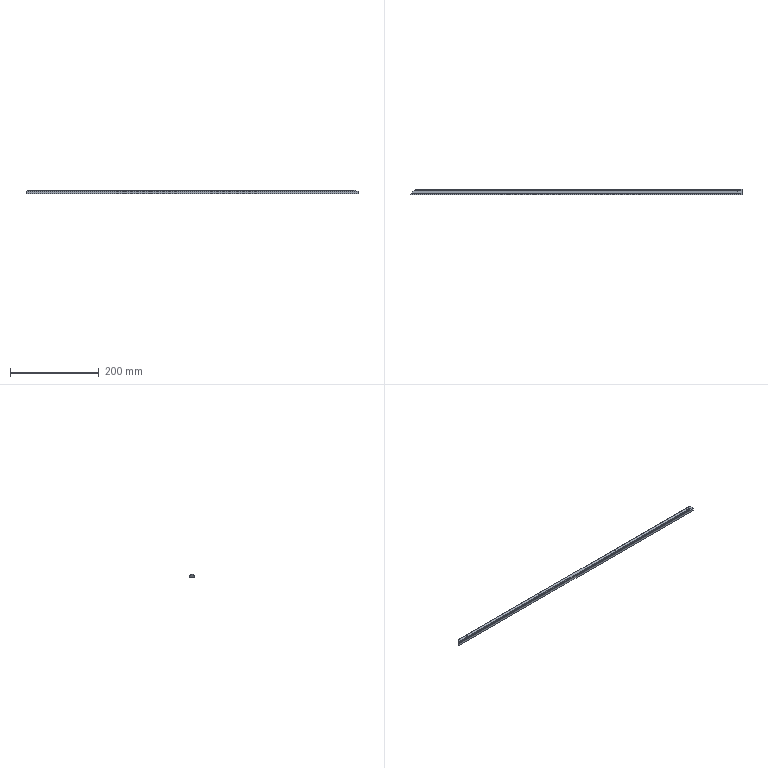Part | STEP file | J013-EBZ05-07-06 | 1 solid | 41 faces | box 748 x 12 x 8 mm | volume 60789 mm3 | plane 17 | cylinder 16 | cone 8 | commonest cylinder face diameters 3.24 x8 4 x8
STEP:
#1=CARTESIAN_POINT('',(257.5,6.,7.835));
#2=VERTEX_POINT('',#1);
#3=CARTESIAN_POINT('',(259.12,6.,6.9));
#4=VERTEX_POINT('',#3);
#5=CARTESIAN_POINT('',(259.12,6.,6.9));
#6=DIRECTION('',(0.866,0.,-0.5));
#7=VECTOR('',#6,1000.);
#8=LINE('',#5,#7);
#9=EDGE_CURVE('',#2,#4,#8,.T.);
#10=ORIENTED_EDGE('',*,*,#9,.F.);
#11=CARTESIAN_POINT('',(255.88,6.,6.9));
#12=VERTEX_POINT('',#11);
#13=CARTESIAN_POINT('',(255.88,6.,6.9));
#14=DIRECTION('',(-0.866,0.,-0.5));
#15=VECTOR('',#14,1000.);
#16=LINE('',#13,#15);
#17=EDGE_CURVE('',#2,#12,#16,.T.);
#18=ORIENTED_EDGE('',*,*,#17,.T.);
#19=CARTESIAN_POINT('',(257.5,6.,6.9));
#20=DIRECTION('',(0.,0.,-1.));
#21=DIRECTION('',(1.,0.,0.));
#22=AXIS2_PLACEMENT_3D('',#19,#20,#21);
#23=CIRCLE('',#22,1.62);
#24=EDGE_CURVE('',#12,#4,#23,.T.);
#25=ORIENTED_EDGE('',*,*,#24,.T.);
#26=EDGE_LOOP('',(#10,#18,#25));
#27=FACE_OUTER_BOUND('',#26,.T.);
#28=CARTESIAN_POINT('',(257.5,6.,6.9));
#29=DIRECTION('',(0.,0.,-1.));
#30=DIRECTION('',(1.,0.,0.));
#31=AXIS2_PLACEMENT_3D('',#28,#29,#30);
#32=CONICAL_SURFACE('',#31,1.62,1.047);
#33=ADVANCED_FACE('',(#27),#32,.F.);
#34=ORIENTED_EDGE('',*,*,#24,.F.);
#35=CARTESIAN_POINT('',(255.88,6.,6.));
#36=VERTEX_POINT('',#35);
#37=CARTESIAN_POINT('',(255.88,6.,0.));
#38=DIRECTION('',(0.,0.,-1.));
#39=VECTOR('',#38,1000.);
#40=LINE('',#37,#39);
#41=EDGE_CURVE('',#12,#36,#40,.T.);
#42=ORIENTED_EDGE('',*,*,#41,.T.);
#43=CARTESIAN_POINT('',(259.12,6.,6.));
#44=VERTEX_POINT('',#43);
#45=CARTESIAN_POINT('',(257.5,6.,6.));
#46=DIRECTION('',(0.,0.,-1.));
#47=DIRECTION('',(1.,0.,0.));
#48=AXIS2_PLACEMENT_3D('',#45,#46,#47);
#49=CIRCLE('',#48,1.62);
#50=EDGE_CURVE('',#36,#44,#49,.T.);
#51=ORIENTED_EDGE('',*,*,#50,.T.);
#52=CARTESIAN_POINT('',(259.12,6.,0.));
#53=DIRECTION('',(0.,0.,-1.));
#54=VECTOR('',#53,1000.);
#55=LINE('',#52,#54);
#56=EDGE_CURVE('',#4,#44,#55,.T.);
#57=ORIENTED_EDGE('',*,*,#56,.F.);
#58=EDGE_LOOP('',(#34,#42,#51,#57));
#59=FACE_OUTER_BOUND('',#58,.T.);
#60=CARTESIAN_POINT('',(257.5,6.,0.));
#61=DIRECTION('',(0.,0.,-1.));
#62=DIRECTION('',(1.,0.,0.));
#63=AXIS2_PLACEMENT_3D('',#60,#61,#62);
#64=CYLINDRICAL_SURFACE('',#63,1.62);
#65=ADVANCED_FACE('',(#59),#64,.F.);
#66=CARTESIAN_POINT('',(255.5,6.,6.));
#67=VERTEX_POINT('',#66);
#68=CARTESIAN_POINT('',(259.5,6.,6.));
#69=VERTEX_POINT('',#68);
#70=CARTESIAN_POINT('',(257.5,6.,6.));
#71=DIRECTION('',(0.,0.,-1.));
#72=DIRECTION('',(1.,0.,0.));
#73=AXIS2_PLACEMENT_3D('',#70,#71,#72);
#74=CIRCLE('',#73,2.);
#75=EDGE_CURVE('',#67,#69,#74,.T.);
#76=ORIENTED_EDGE('',*,*,#75,.F.);
#77=CARTESIAN_POINT('',(255.5,6.,0.));
#78=VERTEX_POINT('',#77);
#79=CARTESIAN_POINT('',(255.5,6.,0.));
#80=DIRECTION('',(0.,0.,-1.));
#81=VECTOR('',#80,1000.);
#82=LINE('',#79,#81);
#83=EDGE_CURVE('',#67,#78,#82,.T.);
#84=ORIENTED_EDGE('',*,*,#83,.T.);
#85=CARTESIAN_POINT('',(259.5,6.,0.));
#86=VERTEX_POINT('',#85);
#87=CARTESIAN_POINT('',(257.5,6.,0.));
#88=DIRECTION('',(0.,0.,-1.));
#89=DIRECTION('',(1.,0.,0.));
#90=AXIS2_PLACEMENT_3D('',#87,#88,#89);
#91=CIRCLE('',#90,2.);
#92=EDGE_CURVE('',#78,#86,#91,.T.);
#93=ORIENTED_EDGE('',*,*,#92,.T.);
#94=CARTESIAN_POINT('',(259.5,6.,0.));
#95=DIRECTION('',(0.,0.,-1.));
#96=VECTOR('',#95,1000.);
#97=LINE('',#94,#96);
#98=EDGE_CURVE('',#69,#86,#97,.T.);
#99=ORIENTED_EDGE('',*,*,#98,.F.);
#100=EDGE_LOOP('',(#76,#84,#93,#99));
#101=FACE_OUTER_BOUND('',#100,.T.);
#102=CARTESIAN_POINT('',(257.5,6.,0.));
#103=DIRECTION('',(0.,0.,-1.));
#104=DIRECTION('',(1.,0.,0.));
#105=AXIS2_PLACEMENT_3D('',#102,#103,#104);
#106=CYLINDRICAL_SURFACE('',#105,2.);
#107=ADVANCED_FACE('',(#101),#106,.F.);
#108=CARTESIAN_POINT('',(497.5,6.,7.835));
#109=VERTEX_POINT('',#108);
#110=CARTESIAN_POINT('',(499.12,6.,6.9));
#111=VERTEX_POINT('',#110);
#112=CARTESIAN_POINT('',(499.12,6.,6.9));
#113=DIRECTION('',(0.866,0.,-0.5));
#114=VECTOR('',#113,1000.);
#115=LINE('',#112,#114);
#116=EDGE_CURVE('',#109,#111,#115,.T.);
#117=ORIENTED_EDGE('',*,*,#116,.F.);
#118=CARTESIAN_POINT('',(495.88,6.,6.9));
#119=VERTEX_POINT('',#118);
#120=CARTESIAN_POINT('',(495.88,6.,6.9));
#121=DIRECTION('',(-0.866,0.,-0.5));
#122=VECTOR('',#121,1000.);
#123=LINE('',#120,#122);
#124=EDGE_CURVE('',#109,#119,#123,.T.);
#125=ORIENTED_EDGE('',*,*,#124,.T.);
#126=CARTESIAN_POINT('',(497.5,6.,6.9));
#127=DIRECTION('',(0.,0.,-1.));
#128=DIRECTION('',(1.,0.,0.));
#129=AXIS2_PLACEMENT_3D('',#126,#127,#128);
#130=CIRCLE('',#129,1.62);
#131=EDGE_CURVE('',#119,#111,#130,.T.);
#132=ORIENTED_EDGE('',*,*,#131,.T.);
#133=EDGE_LOOP('',(#117,#125,#132));
#134=FACE_OUTER_BOUND('',#133,.T.);
#135=CARTESIAN_POINT('',(497.5,6.,6.9));
#136=DIRECTION('',(0.,0.,-1.));
#137=DIRECTION('',(1.,0.,0.));
#138=AXIS2_PLACEMENT_3D('',#135,#136,#137);
#139=CONICAL_SURFACE('',#138,1.62,1.047);
#140=ADVANCED_FACE('',(#134),#139,.F.);
#141=ORIENTED_EDGE('',*,*,#131,.F.);
#142=CARTESIAN_POINT('',(495.88,6.,6.));
#143=VERTEX_POINT('',#142);
#144=CARTESIAN_POINT('',(495.88,6.,0.));
#145=DIRECTION('',(0.,0.,-1.));
#146=VECTOR('',#145,1000.);
#147=LINE('',#144,#146);
#148=EDGE_CURVE('',#119,#143,#147,.T.);
#149=ORIENTED_EDGE('',*,*,#148,.T.);
#150=CARTESIAN_POINT('',(499.12,6.,6.));
#151=VERTEX_POINT('',#150);
#152=CARTESIAN_POINT('',(497.5,6.,6.));
#153=DIRECTION('',(0.,0.,-1.));
#154=DIRECTION('',(1.,0.,0.));
#155=AXIS2_PLACEMENT_3D('',#152,#153,#154);
#156=CIRCLE('',#155,1.62);
#157=EDGE_CURVE('',#143,#151,#156,.T.);
#158=ORIENTED_EDGE('',*,*,#157,.T.);
#159=CARTESIAN_POINT('',(499.12,6.,0.));
#160=DIRECTION('',(0.,0.,-1.));
#161=VECTOR('',#160,1000.);
#162=LINE('',#159,#161);
#163=EDGE_CURVE('',#111,#151,#162,.T.);
#164=ORIENTED_EDGE('',*,*,#163,.F.);
#165=EDGE_LOOP('',(#141,#149,#158,#164));
#166=FACE_OUTER_BOUND('',#165,.T.);
#167=CARTESIAN_POINT('',(497.5,6.,0.));
#168=DIRECTION('',(0.,0.,-1.));
#169=DIRECTION('',(1.,0.,0.));
#170=AXIS2_PLACEMENT_3D('',#167,#168,#169);
#171=CYLINDRICAL_SURFACE('',#170,1.62);
#172=ADVANCED_FACE('',(#166),#171,.F.);
#173=CARTESIAN_POINT('',(495.5,6.,6.));
#174=VERTEX_POINT('',#173);
#175=CARTESIAN_POINT('',(499.5,6.,6.));
#176=VERTEX_POINT('',#175);
#177=CARTESIAN_POINT('',(497.5,6.,6.));
#178=DIRECTION('',(0.,0.,-1.));
#179=DIRECTION('',(1.,0.,0.));
#180=AXIS2_PLACEMENT_3D('',#177,#178,#179);
#181=CIRCLE('',#180,2.);
#182=EDGE_CURVE('',#174,#176,#181,.T.);
#183=ORIENTED_EDGE('',*,*,#182,.F.);
#184=CARTESIAN_POINT('',(495.5,6.,0.));
#185=VERTEX_POINT('',#184);
#186=CARTESIAN_POINT('',(495.5,6.,0.));
#187=DIRECTION('',(0.,0.,-1.));
#188=VECTOR('',#187,1000.);
#189=LINE('',#186,#188);
#190=EDGE_CURVE('',#174,#185,#189,.T.);
#191=ORIENTED_EDGE('',*,*,#190,.T.);
#192=CARTESIAN_POINT('',(499.5,6.,0.));
#193=VERTEX_POINT('',#192);
#194=CARTESIAN_POINT('',(497.5,6.,0.));
#195=DIRECTION('',(0.,0.,-1.));
#196=DIRECTION('',(1.,0.,0.));
#197=AXIS2_PLACEMENT_3D('',#194,#195,#196);
#198=CIRCLE('',#197,2.);
#199=EDGE_CURVE('',#185,#193,#198,.T.);
#200=ORIENTED_EDGE('',*,*,#199,.T.);
#201=CARTESIAN_POINT('',(499.5,6.,0.));
#202=DIRECTION('',(0.,0.,-1.));
#203=VECTOR('',#202,1000.);
#204=LINE('',#201,#203);
#205=EDGE_CURVE('',#176,#193,#204,.T.);
#206=ORIENTED_EDGE('',*,*,#205,.F.);
#207=EDGE_LOOP('',(#183,#191,#200,#206));
#208=FACE_OUTER_BOUND('',#207,.T.);
#209=CARTESIAN_POINT('',(497.5,6.,0.));
#210=DIRECTION('',(0.,0.,-1.));
#211=DIRECTION('',(1.,0.,0.));
#212=AXIS2_PLACEMENT_3D('',#209,#210,#211);
#213=CYLINDRICAL_SURFACE('',#212,2.);
#214=ADVANCED_FACE('',(#208),#213,.F.);
#215=CARTESIAN_POINT('',(27.5,6.,7.835));
#216=VERTEX_POINT('',#215);
#217=CARTESIAN_POINT('',(29.12,6.,6.9));
#218=VERTEX_POINT('',#217);
#219=CARTESIAN_POINT('',(29.12,6.,6.9));
#220=DIRECTION('',(0.866,0.,-0.5));
#221=VECTOR('',#220,1000.);
#222=LINE('',#219,#221);
#223=EDGE_CURVE('',#216,#218,#222,.T.);
#224=ORIENTED_EDGE('',*,*,#223,.F.);
#225=CARTESIAN_POINT('',(25.88,6.,6.9));
#226=VERTEX_POINT('',#225);
#227=CARTESIAN_POINT('',(25.88,6.,6.9));
#228=DIRECTION('',(-0.866,0.,-0.5));
#229=VECTOR('',#228,1000.);
#230=LINE('',#227,#229);
#231=EDGE_CURVE('',#216,#226,#230,.T.);
#232=ORIENTED_EDGE('',*,*,#231,.T.);
#233=CARTESIAN_POINT('',(27.5,6.,6.9));
#234=DIRECTION('',(0.,0.,-1.));
#235=DIRECTION('',(1.,0.,0.));
#236=AXIS2_PLACEMENT_3D('',#233,#234,#235);
#237=CIRCLE('',#236,1.62);
#238=EDGE_CURVE('',#226,#218,#237,.T.);
#239=ORIENTED_EDGE('',*,*,#238,.T.);
#240=EDGE_LOOP('',(#224,#232,#239));
#241=FACE_OUTER_BOUND('',#240,.T.);
#242=CARTESIAN_POINT('',(27.5,6.,6.9));
#243=DIRECTION('',(0.,0.,-1.));
#244=DIRECTION('',(1.,0.,0.));
#245=AXIS2_PLACEMENT_3D('',#242,#243,#244);
#246=CONICAL_SURFACE('',#245,1.62,1.047);
#247=ADVANCED_FACE('',(#241),#246,.F.);
#248=ORIENTED_EDGE('',*,*,#238,.F.);
#249=CARTESIAN_POINT('',(25.88,6.,6.));
#250=VERTEX_POINT('',#249);
#251=CARTESIAN_POINT('',(25.88,6.,0.));
#252=DIRECTION('',(0.,0.,-1.));
#253=VECTOR('',#252,1000.);
#254=LINE('',#251,#253);
#255=EDGE_CURVE('',#226,#250,#254,.T.);
#256=ORIENTED_EDGE('',*,*,#255,.T.);
#257=CARTESIAN_POINT('',(29.12,6.,6.));
#258=VERTEX_POINT('',#257);
#259=CARTESIAN_POINT('',(27.5,6.,6.));
#260=DIRECTION('',(0.,0.,-1.));
#261=DIRECTION('',(1.,0.,0.));
#262=AXIS2_PLACEMENT_3D('',#259,#260,#261);
#263=CIRCLE('',#262,1.62);
#264=EDGE_CURVE('',#250,#258,#263,.T.);
#265=ORIENTED_EDGE('',*,*,#264,.T.);
#266=CARTESIAN_POINT('',(29.12,6.,0.));
#267=DIRECTION('',(0.,0.,-1.));
#268=VECTOR('',#267,1000.);
#269=LINE('',#266,#268);
#270=EDGE_CURVE('',#218,#258,#269,.T.);
#271=ORIENTED_EDGE('',*,*,#270,.F.);
#272=EDGE_LOOP('',(#248,#256,#265,#271));
#273=FACE_OUTER_BOUND('',#272,.T.);
#274=CARTESIAN_POINT('',(27.5,6.,0.));
#275=DIRECTION('',(0.,0.,-1.));
#276=DIRECTION('',(1.,0.,0.));
#277=AXIS2_PLACEMENT_3D('',#274,#275,#276);
#278=CYLINDRICAL_SURFACE('',#277,1.62);
#279=ADVANCED_FACE('',(#273),#278,.F.);
#280=CARTESIAN_POINT('',(25.5,6.,6.));
#281=VERTEX_POINT('',#280);
#282=CARTESIAN_POINT('',(29.5,6.,6.));
#283=VERTEX_POINT('',#282);
#284=CARTESIAN_POINT('',(27.5,6.,6.));
#285=DIRECTION('',(0.,0.,-1.));
#286=DIRECTION('',(1.,0.,0.));
#287=AXIS2_PLACEMENT_3D('',#284,#285,#286);
#288=CIRCLE('',#287,2.);
#289=EDGE_CURVE('',#281,#283,#288,.T.);
#290=ORIENTED_EDGE('',*,*,#289,.F.);
#291=CARTESIAN_POINT('',(25.5,6.,0.));
#292=VERTEX_POINT('',#291);
#293=CARTESIAN_POINT('',(25.5,6.,0.));
#294=DIRECTION('',(0.,0.,-1.));
#295=VECTOR('',#294,1000.);
#296=LINE('',#293,#295);
#297=EDGE_CURVE('',#281,#292,#296,.T.);
#298=ORIENTED_EDGE('',*,*,#297,.T.);
#299=CARTESIAN_POINT('',(29.5,6.,0.));
#300=VERTEX_POINT('',#299);
#301=CARTESIAN_POINT('',(27.5,6.,0.));
#302=DIRECTION('',(0.,0.,-1.));
#303=DIRECTION('',(1.,0.,0.));
#304=AXIS2_PLACEMENT_3D('',#301,#302,#303);
#305=CIRCLE('',#304,2.);
#306=EDGE_CURVE('',#292,#300,#305,.T.);
#307=ORIENTED_EDGE('',*,*,#306,.T.);
#308=CARTESIAN_POINT('',(29.5,6.,0.));
#309=DIRECTION('',(0.,0.,-1.));
#310=VECTOR('',#309,1000.);
#311=LINE('',#308,#310);
#312=EDGE_CURVE('',#283,#300,#311,.T.);
#313=ORIENTED_EDGE('',*,*,#312,.F.);
#314=EDGE_LOOP('',(#290,#298,#307,#313));
#315=FACE_OUTER_BOUND('',#314,.T.);
#316=CARTESIAN_POINT('',(27.5,6.,0.));
#317=DIRECTION('',(0.,0.,-1.));
#318=DIRECTION('',(1.,0.,0.));
#319=AXIS2_PLACEMENT_3D('',#316,#317,#318);
#320=CYLINDRICAL_SURFACE('',#319,2.);
#321=ADVANCED_FACE('',(#315),#320,.F.);
#322=CARTESIAN_POINT('',(727.5,6.,7.835));
#323=VERTEX_POINT('',#322);
#324=CARTESIAN_POINT('',(729.12,6.,6.9));
#325=VERTEX_POINT('',#324);
#326=CARTESIAN_POINT('',(729.12,6.,6.9));
#327=DIRECTION('',(0.866,0.,-0.5));
#328=VECTOR('',#327,1000.);
#329=LINE('',#326,#328);
#330=EDGE_CURVE('',#323,#325,#329,.T.);
#331=ORIENTED_EDGE('',*,*,#330,.F.);
#332=CARTESIAN_POINT('',(725.88,6.,6.9));
#333=VERTEX_POINT('',#332);
#334=CARTESIAN_POINT('',(725.88,6.,6.9));
#335=DIRECTION('',(-0.866,0.,-0.5));
#336=VECTOR('',#335,1000.);
#337=LINE('',#334,#336);
#338=EDGE_CURVE('',#323,#333,#337,.T.);
#339=ORIENTED_EDGE('',*,*,#338,.T.);
#340=CARTESIAN_POINT('',(727.5,6.,6.9));
#341=DIRECTION('',(0.,0.,-1.));
#342=DIRECTION('',(1.,0.,0.));
#343=AXIS2_PLACEMENT_3D('',#340,#341,#342);
#344=CIRCLE('',#343,1.62);
#345=EDGE_CURVE('',#333,#325,#344,.T.);
#346=ORIENTED_EDGE('',*,*,#345,.T.);
#347=EDGE_LOOP('',(#331,#339,#346));
#348=FACE_OUTER_BOUND('',#347,.T.);
#349=CARTESIAN_POINT('',(727.5,6.,6.9));
#350=DIRECTION('',(0.,0.,-1.));
#351=DIRECTION('',(1.,0.,0.));
#352=AXIS2_PLACEMENT_3D('',#349,#350,#351);
#353=CONICAL_SURFACE('',#352,1.62,1.047);
#354=ADVANCED_FACE('',(#348),#353,.F.);
#355=ORIENTED_EDGE('',*,*,#345,.F.);
#356=CARTESIAN_POINT('',(725.88,6.,6.));
#357=VERTEX_POINT('',#356);
#358=CARTESIAN_POINT('',(725.88,6.,0.));
#359=DIRECTION('',(0.,0.,-1.));
#360=VECTOR('',#359,1000.);
#361=LINE('',#358,#360);
#362=EDGE_CURVE('',#333,#357,#361,.T.);
#363=ORIENTED_EDGE('',*,*,#362,.T.);
#364=CARTESIAN_POINT('',(729.12,6.,6.));
#365=VERTEX_POINT('',#364);
#366=CARTESIAN_POINT('',(727.5,6.,6.));
#367=DIRECTION('',(0.,0.,-1.));
#368=DIRECTION('',(1.,0.,0.));
#369=AXIS2_PLACEMENT_3D('',#366,#367,#368);
#370=CIRCLE('',#369,1.62);
#371=EDGE_CURVE('',#357,#365,#370,.T.);
#372=ORIENTED_EDGE('',*,*,#371,.T.);
#373=CARTESIAN_POINT('',(729.12,6.,0.));
#374=DIRECTION('',(0.,0.,-1.));
#375=VECTOR('',#374,1000.);
#376=LINE('',#373,#375);
#377=EDGE_CURVE('',#325,#365,#376,.T.);
#378=ORIENTED_EDGE('',*,*,#377,.F.);
#379=EDGE_LOOP('',(#355,#363,#372,#378));
#380=FACE_OUTER_BOUND('',#379,.T.);
#381=CARTESIAN_POINT('',(727.5,6.,0.));
#382=DIRECTION('',(0.,0.,-1.));
#383=DIRECTION('',(1.,0.,0.));
#384=AXIS2_PLACEMENT_3D('',#381,#382,#383);
#385=CYLINDRICAL_SURFACE('',#384,1.62);
#386=ADVANCED_FACE('',(#380),#385,.F.);
#387=CARTESIAN_POINT('',(725.5,6.,6.));
#388=VERTEX_POINT('',#387);
#389=CARTESIAN_POINT('',(729.5,6.,6.));
#390=VERTEX_POINT('',#389);
#391=CARTESIAN_POINT('',(727.5,6.,6.));
#392=DIRECTION('',(0.,0.,-1.));
#393=DIRECTION('',(1.,0.,0.));
#394=AXIS2_PLACEMENT_3D('',#391,#392,#393);
#395=CIRCLE('',#394,2.);
#396=EDGE_CURVE('',#388,#390,#395,.T.);
#397=ORIENTED_EDGE('',*,*,#396,.F.);
#398=CARTESIAN_POINT('',(725.5,6.,0.));
#399=VERTEX_POINT('',#398);
#400=CARTESIAN_POINT('',(725.5,6.,0.));
#401=DIRECTION('',(0.,0.,-1.));
#402=VECTOR('',#401,1000.);
#403=LINE('',#400,#402);
#404=EDGE_CURVE('',#388,#399,#403,.T.);
#405=ORIENTED_EDGE('',*,*,#404,.T.);
#406=CARTESIAN_POINT('',(729.5,6.,0.));
#407=VERTEX_POINT('',#406);
#408=CARTESIAN_POINT('',(727.5,6.,0.));
#409=DIRECTION('',(0.,0.,-1.));
#410=DIRECTION('',(1.,0.,0.));
#411=AXIS2_PLACEMENT_3D('',#408,#409,#410);
#412=CIRCLE('',#411,2.);
#413=EDGE_CURVE('',#399,#407,#412,.T.);
#414=ORIENTED_EDGE('',*,*,#413,.T.);
#415=CARTESIAN_POINT('',(729.5,6.,0.));
#416=DIRECTION('',(0.,0.,-1.));
#417=VECTOR('',#416,1000.);
#418=LINE('',#415,#417);
#419=EDGE_CURVE('',#390,#407,#418,.T.);
#420=ORIENTED_EDGE('',*,*,#419,.F.);
#421=EDGE_LOOP('',(#397,#405,#414,#420));
#422=FACE_OUTER_BOUND('',#421,.T.);
#423=CARTESIAN_POINT('',(727.5,6.,0.));
#424=DIRECTION('',(0.,0.,-1.));
#425=DIRECTION('',(1.,0.,0.));
#426=AXIS2_PLACEMENT_3D('',#423,#424,#425);
#427=CYLINDRICAL_SURFACE('',#426,2.);
#428=ADVANCED_FACE('',(#422),#427,.F.);
#429=CARTESIAN_POINT('',(6.5,12.,5.5));
#430=VERTEX_POINT('',#429);
#431=CARTESIAN_POINT('',(742.5,12.,5.5));
#432=VERTEX_POINT('',#431);
#433=CARTESIAN_POINT('',(-5.5,12.,5.5));
#434=DIRECTION('',(1.,0.,0.));
#435=VECTOR('',#434,1000.);
#436=LINE('',#433,#435);
#437=EDGE_CURVE('',#430,#432,#436,.T.);
#438=ORIENTED_EDGE('',*,*,#437,.F.);
#439=CARTESIAN_POINT('',(3.8,9.3,5.5));
#440=VERTEX_POINT('',#439);
#441=CARTESIAN_POINT('',(-754.641,-749.141,5.5));
#442=DIRECTION('',(-0.7071,-0.7071,0.));
#443=VECTOR('',#442,1000.);
#444=LINE('',#441,#443);
#445=EDGE_CURVE('',#430,#440,#444,.T.);
#446=ORIENTED_EDGE('',*,*,#445,.T.);
#447=CARTESIAN_POINT('',(732.5,9.3,5.5));
#448=VERTEX_POINT('',#447);
#449=CARTESIAN_POINT('',(-5.5,9.3,5.5));
#450=DIRECTION('',(1.,0.,0.));
#451=VECTOR('',#450,1000.);
#452=LINE('',#449,#451);
#453=EDGE_CURVE('',#440,#448,#452,.T.);
#454=ORIENTED_EDGE('',*,*,#453,.T.);
#455=CARTESIAN_POINT('',(742.5,8.5,5.5));
#456=VERTEX_POINT('',#455);
#457=CARTESIAN_POINT('',(-185.364,82.729,5.5));
#458=DIRECTION('',(0.9968,-0.07975,0.));
#459=VECTOR('',#458,1000.);
#460=LINE('',#457,#459);
#461=EDGE_CURVE('',#448,#456,#460,.T.);
#462=ORIENTED_EDGE('',*,*,#461,.T.);
#463=CARTESIAN_POINT('',(742.5,12.,5.5));
#464=DIRECTION('',(0.,-1.,0.));
#465=VECTOR('',#464,1000.);
#466=LINE('',#463,#465);
#467=EDGE_CURVE('',#432,#456,#466,.T.);
#468=ORIENTED_EDGE('',*,*,#467,.F.);
#469=EDGE_LOOP('',(#438,#446,#454,#462,#468));
#470=FACE_OUTER_BOUND('',#469,.T.);
#471=CARTESIAN_POINT('',(-289.152,-1214.63,5.5));
#472=DIRECTION('',(0.,0.,-1.));
#473=DIRECTION('',(1.,0.,0.));
#474=AXIS2_PLACEMENT_3D('',#471,#472,#473);
#475=PLANE('',#474);
#476=ADVANCED_FACE('',(#470),#475,.F.);
#477=CARTESIAN_POINT('',(742.5,0.,5.5));
#478=VERTEX_POINT('',#477);
#479=CARTESIAN_POINT('',(-5.5,0.,5.5));
#480=VERTEX_POINT('',#479);
#481=CARTESIAN_POINT('',(742.5,0.,5.5));
#482=DIRECTION('',(-1.,0.,0.));
#483=VECTOR('',#482,1000.);
#484=LINE('',#481,#483);
#485=EDGE_CURVE('',#478,#480,#484,.T.);
#486=ORIENTED_EDGE('',*,*,#485,.T.);
#487=CARTESIAN_POINT('',(-5.5,0.,0.));
#488=VERTEX_POINT('',#487);
#489=CARTESIAN_POINT('',(-5.5,0.,0.));
#490=DIRECTION('',(0.,0.,1.));
#491=VECTOR('',#490,1000.);
#492=LINE('',#489,#491);
#493=EDGE_CURVE('',#488,#480,#492,.T.);
#494=ORIENTED_EDGE('',*,*,#493,.F.);
#495=CARTESIAN_POINT('',(742.5,0.,0.));
#496=VERTEX_POINT('',#495);
#497=CARTESIAN_POINT('',(742.5,0.,0.));
#498=DIRECTION('',(-1.,0.,0.));
#499=VECTOR('',#498,1000.);
#500=LINE('',#497,#499);
#501=EDGE_CURVE('',#496,#488,#500,.T.);
#502=ORIENTED_EDGE('',*,*,#501,.F.);
#503=CARTESIAN_POINT('',(742.5,0.,0.));
#504=DIRECTION('',(0.,0.,1.));
#505=VECTOR('',#504,1000.);
#506=LINE('',#503,#505);
#507=EDGE_CURVE('',#496,#478,#506,.T.);
#508=ORIENTED_EDGE('',*,*,#507,.T.);
#509=EDGE_LOOP('',(#486,#494,#502,#508));
#510=FACE_OUTER_BOUND('',#509,.T.);
#511=CARTESIAN_POINT('',(742.5,0.,0.));
#512=DIRECTION('',(0.,1.,0.));
#513=DIRECTION('',(0.,0.,1.));
#514=AXIS2_PLACEMENT_3D('',#511,#512,#513);
#515=PLANE('',#514);
#516=ADVANCED_FACE('',(#510),#515,.F.);
#517=CARTESIAN_POINT('',(6.5,12.,0.));
#518=VERTEX_POINT('',#517);
#519=CARTESIAN_POINT('',(742.5,12.,0.));
#520=VERTEX_POINT('',#519);
#521=CARTESIAN_POINT('',(-5.5,12.,0.));
#522=DIRECTION('',(1.,0.,0.));
#523=VECTOR('',#522,1000.);
#524=LINE('',#521,#523);
#525=EDGE_CURVE('',#518,#520,#524,.T.);
#526=ORIENTED_EDGE('',*,*,#525,.F.);
#527=CARTESIAN_POINT('',(6.5,12.,-0.001006));
#528=DIRECTION('',(0.,0.,1.));
#529=VECTOR('',#528,1000.);
#530=LINE('',#527,#529);
#531=EDGE_CURVE('',#518,#430,#530,.T.);
#532=ORIENTED_EDGE('',*,*,#531,.T.);
#533=ORIENTED_EDGE('',*,*,#437,.T.);
#534=CARTESIAN_POINT('',(742.5,12.,0.));
#535=DIRECTION('',(0.,0.,1.));
#536=VECTOR('',#535,1000.);
#537=LINE('',#534,#536);
#538=EDGE_CURVE('',#520,#432,#537,.T.);
#539=ORIENTED_EDGE('',*,*,#538,.F.);
#540=EDGE_LOOP('',(#526,#532,#533,#539));
#541=FACE_OUTER_BOUND('',#540,.T.);
#542=CARTESIAN_POINT('',(-5.5,12.,0.));
#543=DIRECTION('',(0.,-1.,0.));
#544=DIRECTION('',(0.,0.,-1.));
#545=AXIS2_PLACEMENT_3D('',#542,#543,#544);
#546=PLANE('',#545);
#547=ADVANCED_FACE('',(#541),#546,.F.);
#548=ORIENTED_EDGE('',*,*,#467,.T.);
#549=CARTESIAN_POINT('',(742.5,3.5,5.5));
#550=VERTEX_POINT('',#549);
#551=CARTESIAN_POINT('',(742.5,12.,5.5));
#552=DIRECTION('',(0.,-1.,0.));
#553=VECTOR('',#552,1000.);
#554=LINE('',#551,#553);
#555=EDGE_CURVE('',#456,#550,#554,.T.);
#556=ORIENTED_EDGE('',*,*,#555,.T.);
#557=CARTESIAN_POINT('',(742.5,12.,5.5));
#558=DIRECTION('',(0.,-1.,0.));
#559=VECTOR('',#558,1000.);
#560=LINE('',#557,#559);
#561=EDGE_CURVE('',#550,#478,#560,.T.);
#562=ORIENTED_EDGE('',*,*,#561,.T.);
#563=ORIENTED_EDGE('',*,*,#507,.F.);
#564=CARTESIAN_POINT('',(742.5,12.,0.));
#565=DIRECTION('',(0.,-1.,0.));
#566=VECTOR('',#565,1000.);
#567=LINE('',#564,#566);
#568=EDGE_CURVE('',#520,#496,#567,.T.);
#569=ORIENTED_EDGE('',*,*,#568,.F.);
#570=ORIENTED_EDGE('',*,*,#538,.T.);
#571=EDGE_LOOP('',(#548,#556,#562,#563,#569,#570));
#572=FACE_OUTER_BOUND('',#571,.T.);
#573=CARTESIAN_POINT('',(742.5,12.,0.));
#574=DIRECTION('',(-1.,0.,0.));
#575=DIRECTION('',(0.,0.,-1.));
#576=AXIS2_PLACEMENT_3D('',#573,#574,#575);
#577=PLANE('',#576);
#578=ADVANCED_FACE('',(#572),#577,.F.);
#579=CARTESIAN_POINT('',(-754.641,-749.141,0.));
#580=DIRECTION('',(-0.7071,-0.7071,0.));
#581=VECTOR('',#580,1000.);
#582=LINE('',#579,#581);
#583=EDGE_CURVE('',#518,#488,#582,.T.);
#584=ORIENTED_EDGE('',*,*,#583,.F.);
#585=ORIENTED_EDGE('',*,*,#525,.T.);
#586=ORIENTED_EDGE('',*,*,#568,.T.);
#587=ORIENTED_EDGE('',*,*,#501,.T.);
#588=EDGE_LOOP('',(#584,#585,#586,#587));
#589=FACE_OUTER_BOUND('',#588,.T.);
#590=CARTESIAN_POINT('',(257.5,6.,0.));
#591=DIRECTION('',(0.,0.,-1.));
#592=DIRECTION('',(1.,0.,0.));
#593=AXIS2_PLACEMENT_3D('',#590,#591,#592);
#594=CIRCLE('',#593,2.);
#595=EDGE_CURVE('',#86,#78,#594,.T.);
#596=ORIENTED_EDGE('',*,*,#595,.F.);
#597=ORIENTED_EDGE('',*,*,#92,.F.);
#598=EDGE_LOOP('',(#596,#597));
#599=FACE_BOUND('',#598,.T.);
#600=CARTESIAN_POINT('',(497.5,6.,0.));
#601=DIRECTION('',(0.,0.,-1.));
#602=DIRECTION('',(1.,0.,0.));
#603=AXIS2_PLACEMENT_3D('',#600,#601,#602);
#604=CIRCLE('',#603,2.);
#605=EDGE_CURVE('',#193,#185,#604,.T.);
#606=ORIENTED_EDGE('',*,*,#605,.F.);
#607=ORIENTED_EDGE('',*,*,#199,.F.);
#608=EDGE_LOOP('',(#606,#607));
#609=FACE_BOUND('',#608,.T.);
#610=CARTESIAN_POINT('',(27.5,6.,0.));
#611=DIRECTION('',(0.,0.,-1.));
#612=DIRECTION('',(1.,0.,0.));
#613=AXIS2_PLACEMENT_3D('',#610,#611,#612);
#614=CIRCLE('',#613,2.);
#615=EDGE_CURVE('',#300,#292,#614,.T.);
#616=ORIENTED_EDGE('',*,*,#615,.F.);
#617=ORIENTED_EDGE('',*,*,#306,.F.);
#618=EDGE_LOOP('',(#616,#617));
#619=FACE_BOUND('',#618,.T.);
#620=CARTESIAN_POINT('',(727.5,6.,0.));
#621=DIRECTION('',(0.,0.,-1.));
#622=DIRECTION('',(1.,0.,0.));
#623=AXIS2_PLACEMENT_3D('',#620,#621,#622);
#624=CIRCLE('',#623,2.);
#625=EDGE_CURVE('',#407,#399,#624,.T.);
#626=ORIENTED_EDGE('',*,*,#625,.F.);
#627=ORIENTED_EDGE('',*,*,#413,.F.);
#628=EDGE_LOOP('',(#626,#627));
#629=FACE_BOUND('',#628,.T.);
#630=CARTESIAN_POINT('',(-289.152,-1214.63,0.));
#631=DIRECTION('',(0.,0.,-1.));
#632=DIRECTION('',(1.,0.,0.));
#633=AXIS2_PLACEMENT_3D('',#630,#631,#632);
#634=PLANE('',#633);
#635=ADVANCED_FACE('',(#589,#599,#609,#619,#629),#634,.T.);
#636=CARTESIAN_POINT('',(732.5,2.7,5.5));
#637=VERTEX_POINT('',#636);
#638=CARTESIAN_POINT('',(-2.8,2.7,5.5));
#639=VERTEX_POINT('',#638);
#640=CARTESIAN_POINT('',(742.5,2.7,5.5));
#641=DIRECTION('',(-1.,0.,0.));
#642=VECTOR('',#641,1000.);
#643=LINE('',#640,#642);
#644=EDGE_CURVE('',#637,#639,#643,.T.);
#645=ORIENTED_EDGE('',*,*,#644,.T.);
#646=CARTESIAN_POINT('',(-754.641,-749.141,5.5));
#647=DIRECTION('',(-0.7071,-0.7071,0.));
#648=VECTOR('',#647,1000.);
#649=LINE('',#646,#648);
#650=EDGE_CURVE('',#639,#480,#649,.T.);
#651=ORIENTED_EDGE('',*,*,#650,.T.);
#652=ORIENTED_EDGE('',*,*,#485,.F.);
#653=ORIENTED_EDGE('',*,*,#561,.F.);
#654=CARTESIAN_POINT('',(-379.422,-86.254,5.5));
#655=DIRECTION('',(-0.9968,-0.07975,0.));
#656=VECTOR('',#655,1000.);
#657=LINE('',#654,#656);
#658=EDGE_CURVE('',#550,#637,#657,.T.);
#659=ORIENTED_EDGE('',*,*,#658,.T.);
#660=EDGE_LOOP('',(#645,#651,#652,#653,#659));
#661=FACE_OUTER_BOUND('',#660,.T.);
#662=CARTESIAN_POINT('',(-289.152,-1214.63,5.5));
#663=DIRECTION('',(0.,0.,-1.));
#664=DIRECTION('',(1.,0.,0.));
#665=AXIS2_PLACEMENT_3D('',#662,#663,#664);
#666=PLANE('',#665);
#667=ADVANCED_FACE('',(#661),#666,.F.);
#668=CARTESIAN_POINT('',(3.8,9.3,8.));
#669=VERTEX_POINT('',#668);
#670=CARTESIAN_POINT('',(3.8,9.3,8.));
#671=DIRECTION('',(0.,0.,-1.));
#672=VECTOR('',#671,1000.);
#673=LINE('',#670,#672);
#674=EDGE_CURVE('',#669,#440,#673,.T.);
#675=ORIENTED_EDGE('',*,*,#674,.F.);
#676=CARTESIAN_POINT('',(732.5,9.3,8.));
#677=VERTEX_POINT('',#676);
#678=CARTESIAN_POINT('',(-5.5,9.3,8.));
#679=DIRECTION('',(1.,0.,0.));
#680=VECTOR('',#679,1000.);
#681=LINE('',#678,#680);
#682=EDGE_CURVE('',#669,#677,#681,.T.);
#683=ORIENTED_EDGE('',*,*,#682,.T.);
#684=CARTESIAN_POINT('',(732.5,9.3,5.5));
#685=DIRECTION('',(0.,0.,-1.));
#686=VECTOR('',#685,1000.);
#687=LINE('',#684,#686);
#688=EDGE_CURVE('',#677,#448,#687,.T.);
#689=ORIENTED_EDGE('',*,*,#688,.T.);
#690=ORIENTED_EDGE('',*,*,#453,.F.);
#691=EDGE_LOOP('',(#675,#683,#689,#690));
#692=FACE_OUTER_BOUND('',#691,.T.);
#693=CARTESIAN_POINT('',(-5.5,9.3,8.));
#694=DIRECTION('',(0.,1.,0.));
#695=DIRECTION('',(0.,0.,1.));
#696=AXIS2_PLACEMENT_3D('',#693,#694,#695);
#697=PLANE('',#696);
#698=ADVANCED_FACE('',(#692),#697,.T.);
#699=CARTESIAN_POINT('',(-2.8,2.7,8.));
#700=VERTEX_POINT('',#699);
#701=CARTESIAN_POINT('',(-2.8,2.7,8.));
#702=DIRECTION('',(0.,0.,1.));
#703=VECTOR('',#702,1000.);
#704=LINE('',#701,#703);
#705=EDGE_CURVE('',#639,#700,#704,.T.);
#706=ORIENTED_EDGE('',*,*,#705,.F.);
#707=ORIENTED_EDGE('',*,*,#644,.F.);
#708=CARTESIAN_POINT('',(732.5,2.7,8.));
#709=VERTEX_POINT('',#708);
#710=CARTESIAN_POINT('',(732.5,2.7,8.));
#711=DIRECTION('',(0.,0.,1.));
#712=VECTOR('',#711,1000.);
#713=LINE('',#710,#712);
#714=EDGE_CURVE('',#637,#709,#713,.T.);
#715=ORIENTED_EDGE('',*,*,#714,.T.);
#716=CARTESIAN_POINT('',(742.5,2.7,8.));
#717=DIRECTION('',(-1.,0.,0.));
#718=VECTOR('',#717,1000.);
#719=LINE('',#716,#718);
#720=EDGE_CURVE('',#709,#700,#719,.T.);
#721=ORIENTED_EDGE('',*,*,#720,.T.);
#722=EDGE_LOOP('',(#706,#707,#715,#721));
#723=FACE_OUTER_BOUND('',#722,.T.);
#724=CARTESIAN_POINT('',(742.5,2.7,8.));
#725=DIRECTION('',(0.,-1.,0.));
#726=DIRECTION('',(0.,0.,-1.));
#727=AXIS2_PLACEMENT_3D('',#724,#725,#726);
#728=PLANE('',#727);
#729=ADVANCED_FACE('',(#723),#728,.T.);
#730=ORIENTED_EDGE('',*,*,#682,.F.);
#731=CARTESIAN_POINT('',(-754.641,-749.141,8.));
#732=DIRECTION('',(-0.7071,-0.7071,0.));
#733=VECTOR('',#732,1000.);
#734=LINE('',#731,#733);
#735=EDGE_CURVE('',#669,#700,#734,.T.);
#736=ORIENTED_EDGE('',*,*,#735,.T.);
#737=ORIENTED_EDGE('',*,*,#720,.F.);
#738=CARTESIAN_POINT('',(733.17,2.754,8.));
#739=VERTEX_POINT('',#738);
#740=CARTESIAN_POINT('',(742.5,3.5,8.));
#741=DIRECTION('',(0.9968,0.07975,0.));
#742=VECTOR('',#741,1000.);
#743=LINE('',#740,#742);
#744=EDGE_CURVE('',#709,#739,#743,.T.);
#745=ORIENTED_EDGE('',*,*,#744,.T.);
#746=CARTESIAN_POINT('',(733.17,9.246,8.));
#747=VERTEX_POINT('',#746);
#748=CARTESIAN_POINT('',(733.17,-1214.629,8.));
#749=DIRECTION('',(0.,1.,0.));
#750=VECTOR('',#749,1000.);
#751=LINE('',#748,#750);
#752=EDGE_CURVE('',#739,#747,#751,.T.);
#753=ORIENTED_EDGE('',*,*,#752,.T.);
#754=CARTESIAN_POINT('',(732.5,9.3,8.));
#755=DIRECTION('',(-0.9968,0.07975,0.));
#756=VECTOR('',#755,1000.);
#757=LINE('',#754,#756);
#758=EDGE_CURVE('',#747,#677,#757,.T.);
#759=ORIENTED_EDGE('',*,*,#758,.T.);
#760=EDGE_LOOP('',(#730,#736,#737,#745,#753,#759));
#761=FACE_OUTER_BOUND('',#760,.T.);
#762=CARTESIAN_POINT('',(-289.152,-1214.629,8.));
#763=DIRECTION('',(0.,0.,-1.));
#764=DIRECTION('',(1.,0.,0.));
#765=AXIS2_PLACEMENT_3D('',#762,#763,#764);
#766=PLANE('',#765);
#767=ADVANCED_FACE('',(#761),#766,.F.);
#768=ORIENTED_EDGE('',*,*,#404,.F.);
#769=CARTESIAN_POINT('',(727.5,6.,6.));
#770=DIRECTION('',(0.,0.,-1.));
#771=DIRECTION('',(1.,0.,0.));
#772=AXIS2_PLACEMENT_3D('',#769,#770,#771);
#773=CIRCLE('',#772,2.);
#774=EDGE_CURVE('',#390,#388,#773,.T.);
#775=ORIENTED_EDGE('',*,*,#774,.F.);
#776=ORIENTED_EDGE('',*,*,#419,.T.);
#777=ORIENTED_EDGE('',*,*,#625,.T.);
#778=EDGE_LOOP('',(#768,#775,#776,#777));
#779=FACE_OUTER_BOUND('',#778,.T.);
#780=CARTESIAN_POINT('',(727.5,6.,0.));
#781=DIRECTION('',(0.,0.,-1.));
#782=DIRECTION('',(1.,0.,0.));
#783=AXIS2_PLACEMENT_3D('',#780,#781,#782);
#784=CYLINDRICAL_SURFACE('',#783,2.);
#785=ADVANCED_FACE('',(#779),#784,.F.);
#786=CARTESIAN_POINT('',(727.5,6.,6.));
#787=DIRECTION('',(0.,0.,-1.));
#788=DIRECTION('',(1.,0.,0.));
#789=AXIS2_PLACEMENT_3D('',#786,#787,#788);
#790=CIRCLE('',#789,1.62);
#791=EDGE_CURVE('',#365,#357,#790,.T.);
#792=ORIENTED_EDGE('',*,*,#791,.F.);
#793=ORIENTED_EDGE('',*,*,#371,.F.);
#794=EDGE_LOOP('',(#792,#793));
#795=FACE_BOUND('',#794,.T.);
#796=ORIENTED_EDGE('',*,*,#774,.T.);
#797=ORIENTED_EDGE('',*,*,#396,.T.);
#798=EDGE_LOOP('',(#796,#797));
#799=FACE_OUTER_BOUND('',#798,.T.);
#800=CARTESIAN_POINT('',(725.5,6.,6.));
#801=DIRECTION('',(0.,0.,1.));
#802=DIRECTION('',(-1.,0.,0.));
#803=AXIS2_PLACEMENT_3D('',#800,#801,#802);
#804=PLANE('',#803);
#805=ADVANCED_FACE('',(#795,#799),#804,.F.);
#806=ORIENTED_EDGE('',*,*,#362,.F.);
#807=CARTESIAN_POINT('',(727.5,6.,6.9));
#808=DIRECTION('',(0.,0.,-1.));
#809=DIRECTION('',(1.,0.,0.));
#810=AXIS2_PLACEMENT_3D('',#807,#808,#809);
#811=CIRCLE('',#810,1.62);
#812=EDGE_CURVE('',#325,#333,#811,.T.);
#813=ORIENTED_EDGE('',*,*,#812,.F.);
#814=ORIENTED_EDGE('',*,*,#377,.T.);
#815=ORIENTED_EDGE('',*,*,#791,.T.);
#816=EDGE_LOOP('',(#806,#813,#814,#815));
#817=FACE_OUTER_BOUND('',#816,.T.);
#818=CARTESIAN_POINT('',(727.5,6.,0.));
#819=DIRECTION('',(0.,0.,-1.));
#820=DIRECTION('',(1.,0.,0.));
#821=AXIS2_PLACEMENT_3D('',#818,#819,#820);
#822=CYLINDRICAL_SURFACE('',#821,1.62);
#823=ADVANCED_FACE('',(#817),#822,.F.);
#824=ORIENTED_EDGE('',*,*,#338,.F.);
#825=ORIENTED_EDGE('',*,*,#330,.T.);
#826=ORIENTED_EDGE('',*,*,#812,.T.);
#827=EDGE_LOOP('',(#824,#825,#826));
#828=FACE_OUTER_BOUND('',#827,.T.);
#829=CARTESIAN_POINT('',(727.5,6.,6.9));
#830=DIRECTION('',(0.,0.,-1.));
#831=DIRECTION('',(1.,0.,0.));
#832=AXIS2_PLACEMENT_3D('',#829,#830,#831);
#833=CONICAL_SURFACE('',#832,1.62,1.047);
#834=ADVANCED_FACE('',(#828),#833,.F.);
#835=ORIENTED_EDGE('',*,*,#758,.F.);
#836=CARTESIAN_POINT('',(732.545,9.296,8.168));
#837=DIRECTION('',(0.9631,-0.07704,-0.258));
#838=VECTOR('',#837,1000.);
#839=LINE('',#836,#838);
#840=EDGE_CURVE('',#747,#456,#839,.T.);
#841=ORIENTED_EDGE('',*,*,#840,.T.);
#842=ORIENTED_EDGE('',*,*,#461,.F.);
#843=ORIENTED_EDGE('',*,*,#688,.F.);
#844=EDGE_LOOP('',(#835,#841,#842,#843));
#845=FACE_OUTER_BOUND('',#844,.T.);
#846=CARTESIAN_POINT('',(732.5,9.3,8.));
#847=DIRECTION('',(0.07975,0.9968,0.));
#848=DIRECTION('',(0.,0.,1.));
#849=AXIS2_PLACEMENT_3D('',#846,#847,#848);
#850=PLANE('',#849);
#851=ADVANCED_FACE('',(#845),#850,.T.);
#852=ORIENTED_EDGE('',*,*,#658,.F.);
#853=CARTESIAN_POINT('',(743.867,3.609,5.134));
#854=DIRECTION('',(-0.9631,-0.07704,0.258));
#855=VECTOR('',#854,1000.);
#856=LINE('',#853,#855);
#857=EDGE_CURVE('',#550,#739,#856,.T.);
#858=ORIENTED_EDGE('',*,*,#857,.T.);
#859=ORIENTED_EDGE('',*,*,#744,.F.);
#860=ORIENTED_EDGE('',*,*,#714,.F.);
#861=EDGE_LOOP('',(#852,#858,#859,#860));
#862=FACE_OUTER_BOUND('',#861,.T.);
#863=CARTESIAN_POINT('',(742.5,3.5,0.));
#864=DIRECTION('',(0.07975,-0.9968,0.));
#865=DIRECTION('',(0.,0.,1.));
#866=AXIS2_PLACEMENT_3D('',#863,#864,#865);
#867=PLANE('',#866);
#868=ADVANCED_FACE('',(#862),#867,.T.);
#869=ORIENTED_EDGE('',*,*,#840,.F.);
#870=ORIENTED_EDGE('',*,*,#752,.F.);
#871=ORIENTED_EDGE('',*,*,#857,.F.);
#872=ORIENTED_EDGE('',*,*,#555,.F.);
#873=EDGE_LOOP('',(#869,#870,#871,#872));
#874=FACE_OUTER_BOUND('',#873,.T.);
#875=CARTESIAN_POINT('',(742.5,12.,5.5));
#876=DIRECTION('',(-0.2588,0.,-0.9659));
#877=DIRECTION('',(0.,-1.,0.));
#878=AXIS2_PLACEMENT_3D('',#875,#876,#877);
#879=PLANE('',#878);
#880=ADVANCED_FACE('',(#874),#879,.F.);
#881=ORIENTED_EDGE('',*,*,#297,.F.);
#882=CARTESIAN_POINT('',(27.5,6.,6.));
#883=DIRECTION('',(0.,0.,-1.));
#884=DIRECTION('',(1.,0.,0.));
#885=AXIS2_PLACEMENT_3D('',#882,#883,#884);
#886=CIRCLE('',#885,2.);
#887=EDGE_CURVE('',#283,#281,#886,.T.);
#888=ORIENTED_EDGE('',*,*,#887,.F.);
#889=ORIENTED_EDGE('',*,*,#312,.T.);
#890=ORIENTED_EDGE('',*,*,#615,.T.);
#891=EDGE_LOOP('',(#881,#888,#889,#890));
#892=FACE_OUTER_BOUND('',#891,.T.);
#893=CARTESIAN_POINT('',(27.5,6.,0.));
#894=DIRECTION('',(0.,0.,-1.));
#895=DIRECTION('',(1.,0.,0.));
#896=AXIS2_PLACEMENT_3D('',#893,#894,#895);
#897=CYLINDRICAL_SURFACE('',#896,2.);
#898=ADVANCED_FACE('',(#892),#897,.F.);
#899=CARTESIAN_POINT('',(27.5,6.,6.));
#900=DIRECTION('',(0.,0.,-1.));
#901=DIRECTION('',(1.,0.,0.));
#902=AXIS2_PLACEMENT_3D('',#899,#900,#901);
#903=CIRCLE('',#902,1.62);
#904=EDGE_CURVE('',#258,#250,#903,.T.);
#905=ORIENTED_EDGE('',*,*,#904,.F.);
#906=ORIENTED_EDGE('',*,*,#264,.F.);
#907=EDGE_LOOP('',(#905,#906));
#908=FACE_BOUND('',#907,.T.);
#909=ORIENTED_EDGE('',*,*,#887,.T.);
#910=ORIENTED_EDGE('',*,*,#289,.T.);
#911=EDGE_LOOP('',(#909,#910));
#912=FACE_OUTER_BOUND('',#911,.T.);
#913=CARTESIAN_POINT('',(25.5,6.,6.));
#914=DIRECTION('',(0.,0.,1.));
#915=DIRECTION('',(-1.,0.,0.));
#916=AXIS2_PLACEMENT_3D('',#913,#914,#915);
#917=PLANE('',#916);
#918=ADVANCED_FACE('',(#908,#912),#917,.F.);
#919=ORIENTED_EDGE('',*,*,#255,.F.);
#920=CARTESIAN_POINT('',(27.5,6.,6.9));
#921=DIRECTION('',(0.,0.,-1.));
#922=DIRECTION('',(1.,0.,0.));
#923=AXIS2_PLACEMENT_3D('',#920,#921,#922);
#924=CIRCLE('',#923,1.62);
#925=EDGE_CURVE('',#218,#226,#924,.T.);
#926=ORIENTED_EDGE('',*,*,#925,.F.);
#927=ORIENTED_EDGE('',*,*,#270,.T.);
#928=ORIENTED_EDGE('',*,*,#904,.T.);
#929=EDGE_LOOP('',(#919,#926,#927,#928));
#930=FACE_OUTER_BOUND('',#929,.T.);
#931=CARTESIAN_POINT('',(27.5,6.,0.));
#932=DIRECTION('',(0.,0.,-1.));
#933=DIRECTION('',(1.,0.,0.));
#934=AXIS2_PLACEMENT_3D('',#931,#932,#933);
#935=CYLINDRICAL_SURFACE('',#934,1.62);
#936=ADVANCED_FACE('',(#930),#935,.F.);
#937=ORIENTED_EDGE('',*,*,#231,.F.);
#938=ORIENTED_EDGE('',*,*,#223,.T.);
#939=ORIENTED_EDGE('',*,*,#925,.T.);
#940=EDGE_LOOP('',(#937,#938,#939));
#941=FACE_OUTER_BOUND('',#940,.T.);
#942=CARTESIAN_POINT('',(27.5,6.,6.9));
#943=DIRECTION('',(0.,0.,-1.));
#944=DIRECTION('',(1.,0.,0.));
#945=AXIS2_PLACEMENT_3D('',#942,#943,#944);
#946=CONICAL_SURFACE('',#945,1.62,1.047);
#947=ADVANCED_FACE('',(#941),#946,.F.);
#948=ORIENTED_EDGE('',*,*,#190,.F.);
#949=CARTESIAN_POINT('',(497.5,6.,6.));
#950=DIRECTION('',(0.,0.,-1.));
#951=DIRECTION('',(1.,0.,0.));
#952=AXIS2_PLACEMENT_3D('',#949,#950,#951);
#953=CIRCLE('',#952,2.);
#954=EDGE_CURVE('',#176,#174,#953,.T.);
#955=ORIENTED_EDGE('',*,*,#954,.F.);
#956=ORIENTED_EDGE('',*,*,#205,.T.);
#957=ORIENTED_EDGE('',*,*,#605,.T.);
#958=EDGE_LOOP('',(#948,#955,#956,#957));
#959=FACE_OUTER_BOUND('',#958,.T.);
#960=CARTESIAN_POINT('',(497.5,6.,0.));
#961=DIRECTION('',(0.,0.,-1.));
#962=DIRECTION('',(1.,0.,0.));
#963=AXIS2_PLACEMENT_3D('',#960,#961,#962);
#964=CYLINDRICAL_SURFACE('',#963,2.);
#965=ADVANCED_FACE('',(#959),#964,.F.);
#966=CARTESIAN_POINT('',(497.5,6.,6.));
#967=DIRECTION('',(0.,0.,-1.));
#968=DIRECTION('',(1.,0.,0.));
#969=AXIS2_PLACEMENT_3D('',#966,#967,#968);
#970=CIRCLE('',#969,1.62);
#971=EDGE_CURVE('',#151,#143,#970,.T.);
#972=ORIENTED_EDGE('',*,*,#971,.F.);
#973=ORIENTED_EDGE('',*,*,#157,.F.);
#974=EDGE_LOOP('',(#972,#973));
#975=FACE_BOUND('',#974,.T.);
#976=ORIENTED_EDGE('',*,*,#954,.T.);
#977=ORIENTED_EDGE('',*,*,#182,.T.);
#978=EDGE_LOOP('',(#976,#977));
#979=FACE_OUTER_BOUND('',#978,.T.);
#980=CARTESIAN_POINT('',(495.5,6.,6.));
#981=DIRECTION('',(0.,0.,1.));
#982=DIRECTION('',(-1.,0.,0.));
#983=AXIS2_PLACEMENT_3D('',#980,#981,#982);
#984=PLANE('',#983);
#985=ADVANCED_FACE('',(#975,#979),#984,.F.);
#986=ORIENTED_EDGE('',*,*,#148,.F.);
#987=CARTESIAN_POINT('',(497.5,6.,6.9));
#988=DIRECTION('',(0.,0.,-1.));
#989=DIRECTION('',(1.,0.,0.));
#990=AXIS2_PLACEMENT_3D('',#987,#988,#989);
#991=CIRCLE('',#990,1.62);
#992=EDGE_CURVE('',#111,#119,#991,.T.);
#993=ORIENTED_EDGE('',*,*,#992,.F.);
#994=ORIENTED_EDGE('',*,*,#163,.T.);
#995=ORIENTED_EDGE('',*,*,#971,.T.);
#996=EDGE_LOOP('',(#986,#993,#994,#995));
#997=FACE_OUTER_BOUND('',#996,.T.);
#998=CARTESIAN_POINT('',(497.5,6.,0.));
#999=DIRECTION('',(0.,0.,-1.));
#1000=DIRECTION('',(1.,0.,0.));
#1001=AXIS2_PLACEMENT_3D('',#998,#999,#1000);
#1002=CYLINDRICAL_SURFACE('',#1001,1.62);
#1003=ADVANCED_FACE('',(#997),#1002,.F.);
#1004=ORIENTED_EDGE('',*,*,#124,.F.);
#1005=ORIENTED_EDGE('',*,*,#116,.T.);
#1006=ORIENTED_EDGE('',*,*,#992,.T.);
#1007=EDGE_LOOP('',(#1004,#1005,#1006));
#1008=FACE_OUTER_BOUND('',#1007,.T.);
#1009=CARTESIAN_POINT('',(497.5,6.,6.9));
#1010=DIRECTION('',(0.,0.,-1.));
#1011=DIRECTION('',(1.,0.,0.));
#1012=AXIS2_PLACEMENT_3D('',#1009,#1010,#1011);
#1013=CONICAL_SURFACE('',#1012,1.62,1.047);
#1014=ADVANCED_FACE('',(#1008),#1013,.F.);
#1015=ORIENTED_EDGE('',*,*,#83,.F.);
#1016=CARTESIAN_POINT('',(257.5,6.,6.));
#1017=DIRECTION('',(0.,0.,-1.));
#1018=DIRECTION('',(1.,0.,0.));
#1019=AXIS2_PLACEMENT_3D('',#1016,#1017,#1018);
#1020=CIRCLE('',#1019,2.);
#1021=EDGE_CURVE('',#69,#67,#1020,.T.);
#1022=ORIENTED_EDGE('',*,*,#1021,.F.);
#1023=ORIENTED_EDGE('',*,*,#98,.T.);
#1024=ORIENTED_EDGE('',*,*,#595,.T.);
#1025=EDGE_LOOP('',(#1015,#1022,#1023,#1024));
#1026=FACE_OUTER_BOUND('',#1025,.T.);
#1027=CARTESIAN_POINT('',(257.5,6.,0.));
#1028=DIRECTION('',(0.,0.,-1.));
#1029=DIRECTION('',(1.,0.,0.));
#1030=AXIS2_PLACEMENT_3D('',#1027,#1028,#1029);
#1031=CYLINDRICAL_SURFACE('',#1030,2.);
#1032=ADVANCED_FACE('',(#1026),#1031,.F.);
#1033=CARTESIAN_POINT('',(257.5,6.,6.));
#1034=DIRECTION('',(0.,0.,-1.));
#1035=DIRECTION('',(1.,0.,0.));
#1036=AXIS2_PLACEMENT_3D('',#1033,#1034,#1035);
#1037=CIRCLE('',#1036,1.62);
#1038=EDGE_CURVE('',#44,#36,#1037,.T.);
#1039=ORIENTED_EDGE('',*,*,#1038,.F.);
#1040=ORIENTED_EDGE('',*,*,#50,.F.);
#1041=EDGE_LOOP('',(#1039,#1040));
#1042=FACE_BOUND('',#1041,.T.);
#1043=ORIENTED_EDGE('',*,*,#1021,.T.);
#1044=ORIENTED_EDGE('',*,*,#75,.T.);
#1045=EDGE_LOOP('',(#1043,#1044));
#1046=FACE_OUTER_BOUND('',#1045,.T.);
#1047=CARTESIAN_POINT('',(255.5,6.,6.));
#1048=DIRECTION('',(0.,0.,1.));
#1049=DIRECTION('',(-1.,0.,0.));
#1050=AXIS2_PLACEMENT_3D('',#1047,#1048,#1049);
#1051=PLANE('',#1050);
#1052=ADVANCED_FACE('',(#1042,#1046),#1051,.F.);
#1053=ORIENTED_EDGE('',*,*,#41,.F.);
#1054=CARTESIAN_POINT('',(257.5,6.,6.9));
#1055=DIRECTION('',(0.,0.,-1.));
#1056=DIRECTION('',(1.,0.,0.));
#1057=AXIS2_PLACEMENT_3D('',#1054,#1055,#1056);
#1058=CIRCLE('',#1057,1.62);
#1059=EDGE_CURVE('',#4,#12,#1058,.T.);
#1060=ORIENTED_EDGE('',*,*,#1059,.F.);
#1061=ORIENTED_EDGE('',*,*,#56,.T.);
#1062=ORIENTED_EDGE('',*,*,#1038,.T.);
#1063=EDGE_LOOP('',(#1053,#1060,#1061,#1062));
#1064=FACE_OUTER_BOUND('',#1063,.T.);
#1065=CARTESIAN_POINT('',(257.5,6.,0.));
#1066=DIRECTION('',(0.,0.,-1.));
#1067=DIRECTION('',(1.,0.,0.));
#1068=AXIS2_PLACEMENT_3D('',#1065,#1066,#1067);
#1069=CYLINDRICAL_SURFACE('',#1068,1.62);
#1070=ADVANCED_FACE('',(#1064),#1069,.F.);
#1071=ORIENTED_EDGE('',*,*,#17,.F.);
#1072=ORIENTED_EDGE('',*,*,#9,.T.);
#1073=ORIENTED_EDGE('',*,*,#1059,.T.);
#1074=EDGE_LOOP('',(#1071,#1072,#1073));
#1075=FACE_OUTER_BOUND('',#1074,.T.);
#1076=CARTESIAN_POINT('',(257.5,6.,6.9));
#1077=DIRECTION('',(0.,0.,-1.));
#1078=DIRECTION('',(1.,0.,0.));
#1079=AXIS2_PLACEMENT_3D('',#1076,#1077,#1078);
#1080=CONICAL_SURFACE('',#1079,1.62,1.047);
#1081=ADVANCED_FACE('',(#1075),#1080,.F.);
#1082=ORIENTED_EDGE('',*,*,#531,.F.);
#1083=ORIENTED_EDGE('',*,*,#583,.T.);
#1084=ORIENTED_EDGE('',*,*,#493,.T.);
#1085=ORIENTED_EDGE('',*,*,#650,.F.);
#1086=ORIENTED_EDGE('',*,*,#705,.T.);
#1087=ORIENTED_EDGE('',*,*,#735,.F.);
#1088=ORIENTED_EDGE('',*,*,#674,.T.);
#1089=ORIENTED_EDGE('',*,*,#445,.F.);
#1090=EDGE_LOOP('',(#1082,#1083,#1084,#1085,#1086,#1087,#1088,#1089));
#1091=FACE_OUTER_BOUND('',#1090,.T.);
#1092=CARTESIAN_POINT('',(-5.5,0.,-0.001006));
#1093=DIRECTION('',(0.7071,-0.7071,0.));
#1094=DIRECTION('',(0.7071,0.7071,0.));
#1095=AXIS2_PLACEMENT_3D('',#1092,#1093,#1094);
#1096=PLANE('',#1095);
#1097=ADVANCED_FACE('',(#1091),#1096,.F.);
#1098=CLOSED_SHELL('',(#33,#65,#107,#140,#172,#214,#247,#279,#321,#354,#386,#428,#476,#516,#547,#578,#635,#667,#698,#729,#767,#785,#805,#823,#834,#851,#868,#880,#898,#918,#936,#947,#965,#985,#1003,#1014,#1032,#1052,#1070,#1081,#1097));
#1099=MANIFOLD_SOLID_BREP('',#1098);
#1100=CARTESIAN_POINT('',(0.,0.,0.));
#1101=DIRECTION('',(0.,0.,1.));
#1102=DIRECTION('',(1.,0.,0.));
#1103=AXIS2_PLACEMENT_3D('',#1100,#1101,#1102);
#1104=(LENGTH_UNIT()NAMED_UNIT(*)SI_UNIT(.MILLI.,.METRE.));
#1105=UNCERTAINTY_MEASURE_WITH_UNIT(LENGTH_MEASURE(0.00001),#1104,'','');
#1106=(NAMED_UNIT(*)PLANE_ANGLE_UNIT()SI_UNIT($,.RADIAN.));
#1107=(NAMED_UNIT(*)SI_UNIT($,.STERADIAN.)SOLID_ANGLE_UNIT());
#1108=(GEOMETRIC_REPRESENTATION_CONTEXT(3)GLOBAL_UNCERTAINTY_ASSIGNED_CONTEXT((#1105))GLOBAL_UNIT_ASSIGNED_CONTEXT((#1104,#1106,#1107))REPRESENTATION_CONTEXT('',''));
#1109=ADVANCED_BREP_SHAPE_REPRESENTATION('',(#1099,#1103),#1108);